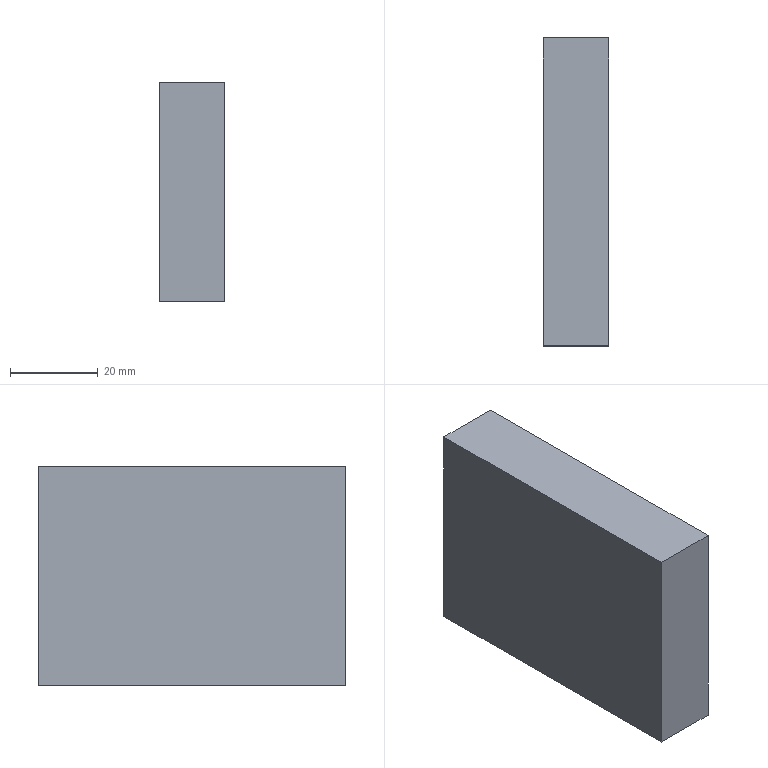Part | STEP file | Tube necking machine_id474_x_t | 1 solid | 6 faces | box 15 x 70 x 50 mm | volume 52500 mm3 | plane 6
STEP:
#1=CARTESIAN_POINT('',(0.,0.,0.));
#2=DIRECTION('',(0.,0.,1.));
#3=DIRECTION('',(1.,0.,0.));
#4=AXIS2_PLACEMENT_3D('',#1,#2,#3);
#5=CARTESIAN_POINT('',(-235.5,15.,166.));
#6=VERTEX_POINT('',#5);
#7=CARTESIAN_POINT('',(-235.5,15.,216.));
#8=VERTEX_POINT('',#7);
#9=CARTESIAN_POINT('',(-235.5,15.,216.));
#10=DIRECTION('',(0.,0.,1.));
#11=VECTOR('',#10,1.);
#12=LINE('',#9,#11);
#13=CARTESIAN_POINT('',(-220.5,15.,216.));
#14=DIRECTION('',(0.,-1.,0.));
#15=DIRECTION('',(0.,0.,-1.));
#16=AXIS2_PLACEMENT_3D('',#13,#14,#15);
#17=PLANE('',#16);
#18=CARTESIAN_POINT('',(0.,-15.));
#19=DIRECTION('',(-1.,0.));
#20=VECTOR('',#19,1.);
#21=LINE('',#18,#20);
#22=(GEOMETRIC_REPRESENTATION_CONTEXT(2)PARAMETRIC_REPRESENTATION_CONTEXT()REPRESENTATION_CONTEXT('',''));
#23=DEFINITIONAL_REPRESENTATION('',(#21),#22);
#24=PCURVE('',#17,#23);
#25=CARTESIAN_POINT('',(-235.5,0.,0.));
#26=DIRECTION('',(-1.,0.,0.));
#27=DIRECTION('',(0.,0.,-1.));
#28=AXIS2_PLACEMENT_3D('',#25,#26,#27);
#29=PLANE('',#28);
#30=CARTESIAN_POINT('',(-216.,-15.));
#31=DIRECTION('',(-1.,0.));
#32=VECTOR('',#31,1.);
#33=LINE('',#30,#32);
#34=(GEOMETRIC_REPRESENTATION_CONTEXT(2)PARAMETRIC_REPRESENTATION_CONTEXT()REPRESENTATION_CONTEXT('',''));
#35=DEFINITIONAL_REPRESENTATION('',(#33),#34);
#36=PCURVE('',#29,#35);
#37=SURFACE_CURVE('',#12,(#24,#36),.PCURVE_S1.);
#38=EDGE_CURVE('',#6,#8,#37,.T.);
#39=ORIENTED_EDGE('',*,*,#38,.F.);
#40=CARTESIAN_POINT('',(-220.5,15.,166.));
#41=VERTEX_POINT('',#40);
#42=CARTESIAN_POINT('',(-220.5,15.,166.));
#43=DIRECTION('',(1.,0.,0.));
#44=VECTOR('',#43,1.);
#45=LINE('',#42,#44);
#46=CARTESIAN_POINT('',(50.,0.));
#47=DIRECTION('',(0.,1.));
#48=VECTOR('',#47,1.);
#49=LINE('',#46,#48);
#50=(GEOMETRIC_REPRESENTATION_CONTEXT(2)PARAMETRIC_REPRESENTATION_CONTEXT()REPRESENTATION_CONTEXT('',''));
#51=DEFINITIONAL_REPRESENTATION('',(#49),#50);
#52=PCURVE('',#17,#51);
#53=CARTESIAN_POINT('',(-220.5,15.,166.));
#54=DIRECTION('',(0.,0.,-1.));
#55=DIRECTION('',(1.,0.,0.));
#56=AXIS2_PLACEMENT_3D('',#53,#54,#55);
#57=PLANE('',#56);
#58=CARTESIAN_POINT('',(0.,0.));
#59=DIRECTION('',(1.,0.));
#60=VECTOR('',#59,1.);
#61=LINE('',#58,#60);
#62=(GEOMETRIC_REPRESENTATION_CONTEXT(2)PARAMETRIC_REPRESENTATION_CONTEXT()REPRESENTATION_CONTEXT('',''));
#63=DEFINITIONAL_REPRESENTATION('',(#61),#62);
#64=PCURVE('',#57,#63);
#65=SURFACE_CURVE('',#45,(#52,#64),.PCURVE_S1.);
#66=EDGE_CURVE('',#6,#41,#65,.T.);
#67=ORIENTED_EDGE('',*,*,#66,.T.);
#68=CARTESIAN_POINT('',(-220.5,15.,216.));
#69=VERTEX_POINT('',#68);
#70=CARTESIAN_POINT('',(-220.5,15.,216.));
#71=DIRECTION('',(0.,0.,1.));
#72=VECTOR('',#71,1.);
#73=LINE('',#70,#72);
#74=CARTESIAN_POINT('',(0.,0.));
#75=DIRECTION('',(-1.,0.));
#76=VECTOR('',#75,1.);
#77=LINE('',#74,#76);
#78=(GEOMETRIC_REPRESENTATION_CONTEXT(2)PARAMETRIC_REPRESENTATION_CONTEXT()REPRESENTATION_CONTEXT('',''));
#79=DEFINITIONAL_REPRESENTATION('',(#77),#78);
#80=PCURVE('',#17,#79);
#81=CARTESIAN_POINT('',(-220.5,0.,0.));
#82=DIRECTION('',(-1.,0.,0.));
#83=DIRECTION('',(0.,0.,-1.));
#84=AXIS2_PLACEMENT_3D('',#81,#82,#83);
#85=PLANE('',#84);
#86=CARTESIAN_POINT('',(-216.,-15.));
#87=DIRECTION('',(-1.,0.));
#88=VECTOR('',#87,1.);
#89=LINE('',#86,#88);
#90=(GEOMETRIC_REPRESENTATION_CONTEXT(2)PARAMETRIC_REPRESENTATION_CONTEXT()REPRESENTATION_CONTEXT('',''));
#91=DEFINITIONAL_REPRESENTATION('',(#89),#90);
#92=PCURVE('',#85,#91);
#93=SURFACE_CURVE('',#73,(#80,#92),.PCURVE_S1.);
#94=EDGE_CURVE('',#41,#69,#93,.T.);
#95=ORIENTED_EDGE('',*,*,#94,.T.);
#96=CARTESIAN_POINT('',(-220.5,15.,216.));
#97=DIRECTION('',(1.,0.,0.));
#98=VECTOR('',#97,1.);
#99=LINE('',#96,#98);
#100=CARTESIAN_POINT('',(0.,0.));
#101=DIRECTION('',(0.,1.));
#102=VECTOR('',#101,1.);
#103=LINE('',#100,#102);
#104=(GEOMETRIC_REPRESENTATION_CONTEXT(2)PARAMETRIC_REPRESENTATION_CONTEXT()REPRESENTATION_CONTEXT('',''));
#105=DEFINITIONAL_REPRESENTATION('',(#103),#104);
#106=PCURVE('',#17,#105);
#107=CARTESIAN_POINT('',(-220.5,85.,216.));
#108=DIRECTION('',(0.,0.,1.));
#109=DIRECTION('',(-1.,0.,0.));
#110=AXIS2_PLACEMENT_3D('',#107,#108,#109);
#111=PLANE('',#110);
#112=CARTESIAN_POINT('',(0.,70.));
#113=DIRECTION('',(-1.,0.));
#114=VECTOR('',#113,1.);
#115=LINE('',#112,#114);
#116=(GEOMETRIC_REPRESENTATION_CONTEXT(2)PARAMETRIC_REPRESENTATION_CONTEXT()REPRESENTATION_CONTEXT('',''));
#117=DEFINITIONAL_REPRESENTATION('',(#115),#116);
#118=PCURVE('',#111,#117);
#119=SURFACE_CURVE('',#99,(#106,#118),.PCURVE_S1.);
#120=EDGE_CURVE('',#8,#69,#119,.T.);
#121=ORIENTED_EDGE('',*,*,#120,.F.);
#122=EDGE_LOOP('',(#39,#67,#95,#121));
#123=FACE_BOUND('',#122,.T.);
#124=ADVANCED_FACE('',(#123),#17,.T.);
#125=CARTESIAN_POINT('',(-235.5,85.,166.));
#126=VERTEX_POINT('',#125);
#127=CARTESIAN_POINT('',(-235.5,15.,166.));
#128=DIRECTION('',(0.,-1.,0.));
#129=VECTOR('',#128,1.);
#130=LINE('',#127,#129);
#131=CARTESIAN_POINT('',(-15.,0.));
#132=DIRECTION('',(0.,1.));
#133=VECTOR('',#132,1.);
#134=LINE('',#131,#133);
#135=(GEOMETRIC_REPRESENTATION_CONTEXT(2)PARAMETRIC_REPRESENTATION_CONTEXT()REPRESENTATION_CONTEXT('',''));
#136=DEFINITIONAL_REPRESENTATION('',(#134),#135);
#137=PCURVE('',#57,#136);
#138=CARTESIAN_POINT('',(-166.,-15.));
#139=DIRECTION('',(0.,1.));
#140=VECTOR('',#139,1.);
#141=LINE('',#138,#140);
#142=(GEOMETRIC_REPRESENTATION_CONTEXT(2)PARAMETRIC_REPRESENTATION_CONTEXT()REPRESENTATION_CONTEXT('',''));
#143=DEFINITIONAL_REPRESENTATION('',(#141),#142);
#144=PCURVE('',#29,#143);
#145=SURFACE_CURVE('',#130,(#137,#144),.PCURVE_S1.);
#146=EDGE_CURVE('',#126,#6,#145,.T.);
#147=ORIENTED_EDGE('',*,*,#146,.F.);
#148=CARTESIAN_POINT('',(-220.5,85.,166.));
#149=VERTEX_POINT('',#148);
#150=CARTESIAN_POINT('',(-220.5,85.,166.));
#151=DIRECTION('',(1.,0.,0.));
#152=VECTOR('',#151,1.);
#153=LINE('',#150,#152);
#154=CARTESIAN_POINT('',(0.,-70.));
#155=DIRECTION('',(1.,0.));
#156=VECTOR('',#155,1.);
#157=LINE('',#154,#156);
#158=(GEOMETRIC_REPRESENTATION_CONTEXT(2)PARAMETRIC_REPRESENTATION_CONTEXT()REPRESENTATION_CONTEXT('',''));
#159=DEFINITIONAL_REPRESENTATION('',(#157),#158);
#160=PCURVE('',#57,#159);
#161=CARTESIAN_POINT('',(-220.5,85.,166.));
#162=DIRECTION('',(0.,1.,0.));
#163=DIRECTION('',(0.,0.,1.));
#164=AXIS2_PLACEMENT_3D('',#161,#162,#163);
#165=PLANE('',#164);
#166=CARTESIAN_POINT('',(0.,0.));
#167=DIRECTION('',(0.,1.));
#168=VECTOR('',#167,1.);
#169=LINE('',#166,#168);
#170=(GEOMETRIC_REPRESENTATION_CONTEXT(2)PARAMETRIC_REPRESENTATION_CONTEXT()REPRESENTATION_CONTEXT('',''));
#171=DEFINITIONAL_REPRESENTATION('',(#169),#170);
#172=PCURVE('',#165,#171);
#173=SURFACE_CURVE('',#153,(#160,#172),.PCURVE_S1.);
#174=EDGE_CURVE('',#126,#149,#173,.T.);
#175=ORIENTED_EDGE('',*,*,#174,.T.);
#176=CARTESIAN_POINT('',(-220.5,15.,166.));
#177=DIRECTION('',(0.,-1.,0.));
#178=VECTOR('',#177,1.);
#179=LINE('',#176,#178);
#180=CARTESIAN_POINT('',(0.,0.));
#181=DIRECTION('',(0.,1.));
#182=VECTOR('',#181,1.);
#183=LINE('',#180,#182);
#184=(GEOMETRIC_REPRESENTATION_CONTEXT(2)PARAMETRIC_REPRESENTATION_CONTEXT()REPRESENTATION_CONTEXT('',''));
#185=DEFINITIONAL_REPRESENTATION('',(#183),#184);
#186=PCURVE('',#57,#185);
#187=CARTESIAN_POINT('',(-166.,-15.));
#188=DIRECTION('',(0.,1.));
#189=VECTOR('',#188,1.);
#190=LINE('',#187,#189);
#191=(GEOMETRIC_REPRESENTATION_CONTEXT(2)PARAMETRIC_REPRESENTATION_CONTEXT()REPRESENTATION_CONTEXT('',''));
#192=DEFINITIONAL_REPRESENTATION('',(#190),#191);
#193=PCURVE('',#85,#192);
#194=SURFACE_CURVE('',#179,(#186,#193),.PCURVE_S1.);
#195=EDGE_CURVE('',#149,#41,#194,.T.);
#196=ORIENTED_EDGE('',*,*,#195,.T.);
#197=ORIENTED_EDGE('',*,*,#66,.F.);
#198=EDGE_LOOP('',(#147,#175,#196,#197));
#199=FACE_BOUND('',#198,.T.);
#200=ADVANCED_FACE('',(#199),#57,.T.);
#201=CARTESIAN_POINT('',(-235.5,85.,216.));
#202=VERTEX_POINT('',#201);
#203=CARTESIAN_POINT('',(-235.5,85.,166.));
#204=DIRECTION('',(0.,0.,-1.));
#205=VECTOR('',#204,1.);
#206=LINE('',#203,#205);
#207=CARTESIAN_POINT('',(0.,-15.));
#208=DIRECTION('',(-1.,0.));
#209=VECTOR('',#208,1.);
#210=LINE('',#207,#209);
#211=(GEOMETRIC_REPRESENTATION_CONTEXT(2)PARAMETRIC_REPRESENTATION_CONTEXT()REPRESENTATION_CONTEXT('',''));
#212=DEFINITIONAL_REPRESENTATION('',(#210),#211);
#213=PCURVE('',#165,#212);
#214=CARTESIAN_POINT('',(-166.,-85.));
#215=DIRECTION('',(1.,0.));
#216=VECTOR('',#215,1.);
#217=LINE('',#214,#216);
#218=(GEOMETRIC_REPRESENTATION_CONTEXT(2)PARAMETRIC_REPRESENTATION_CONTEXT()REPRESENTATION_CONTEXT('',''));
#219=DEFINITIONAL_REPRESENTATION('',(#217),#218);
#220=PCURVE('',#29,#219);
#221=SURFACE_CURVE('',#206,(#213,#220),.PCURVE_S1.);
#222=EDGE_CURVE('',#202,#126,#221,.T.);
#223=ORIENTED_EDGE('',*,*,#222,.F.);
#224=CARTESIAN_POINT('',(-220.5,85.,216.));
#225=VERTEX_POINT('',#224);
#226=CARTESIAN_POINT('',(-220.5,85.,216.));
#227=DIRECTION('',(1.,0.,0.));
#228=VECTOR('',#227,1.);
#229=LINE('',#226,#228);
#230=CARTESIAN_POINT('',(50.,0.));
#231=DIRECTION('',(0.,1.));
#232=VECTOR('',#231,1.);
#233=LINE('',#230,#232);
#234=(GEOMETRIC_REPRESENTATION_CONTEXT(2)PARAMETRIC_REPRESENTATION_CONTEXT()REPRESENTATION_CONTEXT('',''));
#235=DEFINITIONAL_REPRESENTATION('',(#233),#234);
#236=PCURVE('',#165,#235);
#237=CARTESIAN_POINT('',(0.,0.));
#238=DIRECTION('',(-1.,0.));
#239=VECTOR('',#238,1.);
#240=LINE('',#237,#239);
#241=(GEOMETRIC_REPRESENTATION_CONTEXT(2)PARAMETRIC_REPRESENTATION_CONTEXT()REPRESENTATION_CONTEXT('',''));
#242=DEFINITIONAL_REPRESENTATION('',(#240),#241);
#243=PCURVE('',#111,#242);
#244=SURFACE_CURVE('',#229,(#236,#243),.PCURVE_S1.);
#245=EDGE_CURVE('',#202,#225,#244,.T.);
#246=ORIENTED_EDGE('',*,*,#245,.T.);
#247=CARTESIAN_POINT('',(-220.5,85.,166.));
#248=DIRECTION('',(0.,0.,-1.));
#249=VECTOR('',#248,1.);
#250=LINE('',#247,#249);
#251=CARTESIAN_POINT('',(0.,0.));
#252=DIRECTION('',(-1.,0.));
#253=VECTOR('',#252,1.);
#254=LINE('',#251,#253);
#255=(GEOMETRIC_REPRESENTATION_CONTEXT(2)PARAMETRIC_REPRESENTATION_CONTEXT()REPRESENTATION_CONTEXT('',''));
#256=DEFINITIONAL_REPRESENTATION('',(#254),#255);
#257=PCURVE('',#165,#256);
#258=CARTESIAN_POINT('',(-166.,-85.));
#259=DIRECTION('',(1.,0.));
#260=VECTOR('',#259,1.);
#261=LINE('',#258,#260);
#262=(GEOMETRIC_REPRESENTATION_CONTEXT(2)PARAMETRIC_REPRESENTATION_CONTEXT()REPRESENTATION_CONTEXT('',''));
#263=DEFINITIONAL_REPRESENTATION('',(#261),#262);
#264=PCURVE('',#85,#263);
#265=SURFACE_CURVE('',#250,(#257,#264),.PCURVE_S1.);
#266=EDGE_CURVE('',#225,#149,#265,.T.);
#267=ORIENTED_EDGE('',*,*,#266,.T.);
#268=ORIENTED_EDGE('',*,*,#174,.F.);
#269=EDGE_LOOP('',(#223,#246,#267,#268));
#270=FACE_BOUND('',#269,.T.);
#271=ADVANCED_FACE('',(#270),#165,.T.);
#272=CARTESIAN_POINT('',(-235.5,85.,216.));
#273=DIRECTION('',(0.,1.,0.));
#274=VECTOR('',#273,1.);
#275=LINE('',#272,#274);
#276=CARTESIAN_POINT('',(15.,0.));
#277=DIRECTION('',(0.,-1.));
#278=VECTOR('',#277,1.);
#279=LINE('',#276,#278);
#280=(GEOMETRIC_REPRESENTATION_CONTEXT(2)PARAMETRIC_REPRESENTATION_CONTEXT()REPRESENTATION_CONTEXT('',''));
#281=DEFINITIONAL_REPRESENTATION('',(#279),#280);
#282=PCURVE('',#111,#281);
#283=CARTESIAN_POINT('',(-216.,-85.));
#284=DIRECTION('',(0.,-1.));
#285=VECTOR('',#284,1.);
#286=LINE('',#283,#285);
#287=(GEOMETRIC_REPRESENTATION_CONTEXT(2)PARAMETRIC_REPRESENTATION_CONTEXT()REPRESENTATION_CONTEXT('',''));
#288=DEFINITIONAL_REPRESENTATION('',(#286),#287);
#289=PCURVE('',#29,#288);
#290=SURFACE_CURVE('',#275,(#282,#289),.PCURVE_S1.);
#291=EDGE_CURVE('',#8,#202,#290,.T.);
#292=ORIENTED_EDGE('',*,*,#291,.F.);
#293=ORIENTED_EDGE('',*,*,#120,.T.);
#294=CARTESIAN_POINT('',(-220.5,85.,216.));
#295=DIRECTION('',(0.,1.,0.));
#296=VECTOR('',#295,1.);
#297=LINE('',#294,#296);
#298=CARTESIAN_POINT('',(0.,0.));
#299=DIRECTION('',(0.,-1.));
#300=VECTOR('',#299,1.);
#301=LINE('',#298,#300);
#302=(GEOMETRIC_REPRESENTATION_CONTEXT(2)PARAMETRIC_REPRESENTATION_CONTEXT()REPRESENTATION_CONTEXT('',''));
#303=DEFINITIONAL_REPRESENTATION('',(#301),#302);
#304=PCURVE('',#111,#303);
#305=CARTESIAN_POINT('',(-216.,-85.));
#306=DIRECTION('',(0.,-1.));
#307=VECTOR('',#306,1.);
#308=LINE('',#305,#307);
#309=(GEOMETRIC_REPRESENTATION_CONTEXT(2)PARAMETRIC_REPRESENTATION_CONTEXT()REPRESENTATION_CONTEXT('',''));
#310=DEFINITIONAL_REPRESENTATION('',(#308),#309);
#311=PCURVE('',#85,#310);
#312=SURFACE_CURVE('',#297,(#304,#311),.PCURVE_S1.);
#313=EDGE_CURVE('',#69,#225,#312,.T.);
#314=ORIENTED_EDGE('',*,*,#313,.T.);
#315=ORIENTED_EDGE('',*,*,#245,.F.);
#316=EDGE_LOOP('',(#292,#293,#314,#315));
#317=FACE_BOUND('',#316,.T.);
#318=ADVANCED_FACE('',(#317),#111,.T.);
#319=ORIENTED_EDGE('',*,*,#94,.F.);
#320=ORIENTED_EDGE('',*,*,#195,.F.);
#321=ORIENTED_EDGE('',*,*,#266,.F.);
#322=ORIENTED_EDGE('',*,*,#313,.F.);
#323=EDGE_LOOP('',(#319,#320,#321,#322));
#324=FACE_BOUND('',#323,.T.);
#325=ADVANCED_FACE('',(#324),#85,.F.);
#326=ORIENTED_EDGE('',*,*,#38,.T.);
#327=ORIENTED_EDGE('',*,*,#291,.T.);
#328=ORIENTED_EDGE('',*,*,#222,.T.);
#329=ORIENTED_EDGE('',*,*,#146,.T.);
#330=EDGE_LOOP('',(#326,#327,#328,#329));
#331=FACE_BOUND('',#330,.T.);
#332=ADVANCED_FACE('',(#331),#29,.T.);
#333=CLOSED_SHELL('',(#124,#200,#271,#318,#325,#332));
#334=MANIFOLD_SOLID_BREP('',#333);
#335=(LENGTH_UNIT()NAMED_UNIT(*)SI_UNIT(.MILLI.,.METRE.));
#336=UNCERTAINTY_MEASURE_WITH_UNIT(LENGTH_MEASURE(0.0000001),#335,'','');
#337=(NAMED_UNIT(*)PLANE_ANGLE_UNIT()SI_UNIT($,.RADIAN.));
#338=(NAMED_UNIT(*)SI_UNIT($,.STERADIAN.)SOLID_ANGLE_UNIT());
#339=(GEOMETRIC_REPRESENTATION_CONTEXT(3)GLOBAL_UNCERTAINTY_ASSIGNED_CONTEXT((#336))GLOBAL_UNIT_ASSIGNED_CONTEXT((#335,#337,#338))REPRESENTATION_CONTEXT('',''));
#340=ADVANCED_BREP_SHAPE_REPRESENTATION('',(#4,#334),#339);